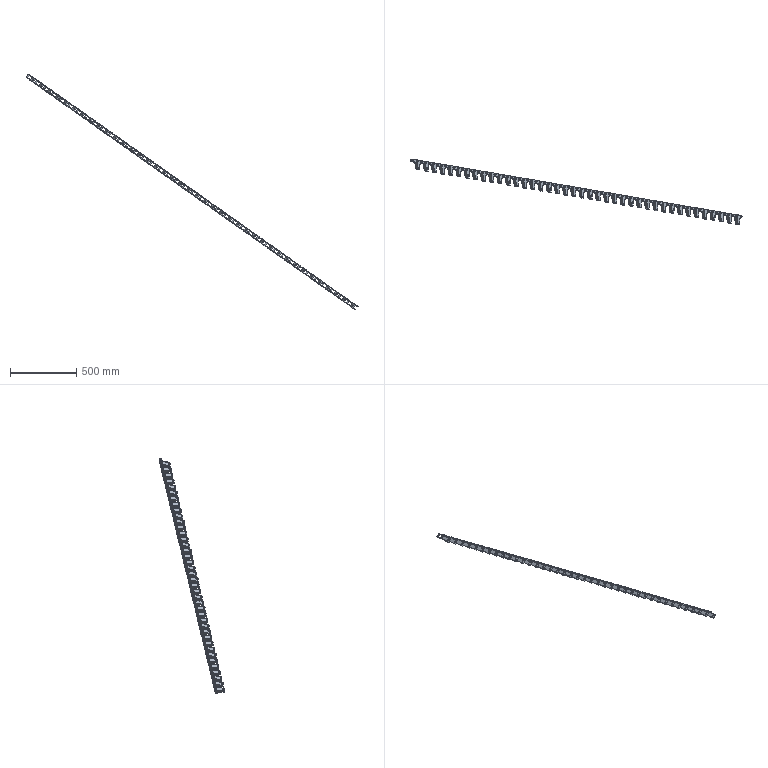Part | STEP file | right conveyor single-link chain | 80 solids | 2080 faces | box 2497 x 489.718 x 1775 mm | volume 773582 mm3 | plane 1120 | cylinder 960 | commonest cylinder face diameters 6 x320 18 x320 20 x120 4 x80 12 x80 16 x40